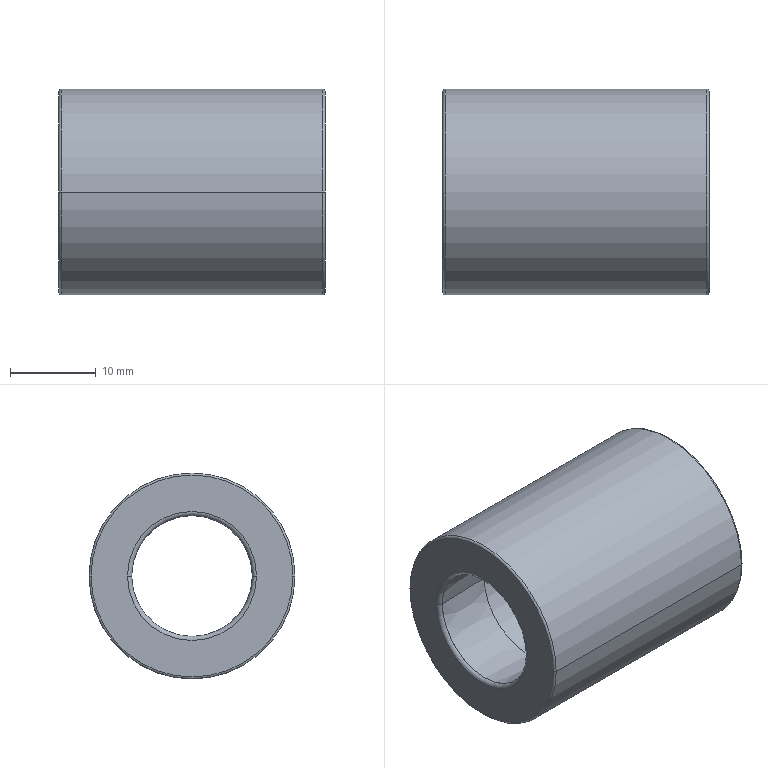Part | NX | 1 solid | 26 faces | box 31 x 24 x 24 mm | volume 8171 mm3 | torus 12 | cone 8 | cylinder 4 | plane 2 | commonest cylinder face diameters 16.674 x2 24 x2
STEP:
#1=CARTESIAN_POINT('',(-7.257,8.337,0.));
#2=VERTEX_POINT('',#1);
#3=CARTESIAN_POINT('',(-7.257,-8.337,0.));
#4=VERTEX_POINT('',#3);
#5=CARTESIAN_POINT('',(-7.257,0.,0.));
#6=DIRECTION('',(-1.,0.,0.));
#7=DIRECTION('',(0.,-1.,0.));
#8=AXIS2_PLACEMENT_3D('',#5,#6,#7);
#9=CIRCLE('',#8,8.337);
#10=EDGE_CURVE('',#2,#4,#9,.T.);
#11=ORIENTED_EDGE('',*,*,#10,.T.);
#12=CARTESIAN_POINT('',(7.257,-8.337,0.));
#13=VERTEX_POINT('',#12);
#14=CARTESIAN_POINT('',(0.,-8.337,0.));
#15=DIRECTION('',(1.,0.,0.));
#16=VECTOR('',#15,1000.);
#17=LINE('',#14,#16);
#18=EDGE_CURVE('',#4,#13,#17,.T.);
#19=ORIENTED_EDGE('',*,*,#18,.T.);
#20=CARTESIAN_POINT('',(7.257,8.337,0.));
#21=VERTEX_POINT('',#20);
#22=CARTESIAN_POINT('',(7.257,0.,0.));
#23=DIRECTION('',(1.,0.,0.));
#24=DIRECTION('',(0.,-1.,0.));
#25=AXIS2_PLACEMENT_3D('',#22,#23,#24);
#26=CIRCLE('',#25,8.337);
#27=EDGE_CURVE('',#13,#21,#26,.T.);
#28=ORIENTED_EDGE('',*,*,#27,.T.);
#29=CARTESIAN_POINT('',(0.,8.337,0.));
#30=DIRECTION('',(1.,0.,0.));
#31=VECTOR('',#30,1000.);
#32=LINE('',#29,#31);
#33=EDGE_CURVE('',#2,#21,#32,.T.);
#34=ORIENTED_EDGE('',*,*,#33,.F.);
#35=EDGE_LOOP('',(#11,#19,#28,#34));
#36=FACE_BOUND('',#35,.T.);
#37=CARTESIAN_POINT('',(0.,0.,0.));
#38=DIRECTION('',(1.,0.,0.));
#39=DIRECTION('',(0.,1.,0.));
#40=AXIS2_PLACEMENT_3D('',#37,#38,#39);
#41=CYLINDRICAL_SURFACE('',#40,8.337);
#42=ADVANCED_FACE('',(#36),#41,.F.);
#43=CARTESIAN_POINT('',(-15.02,7.033,0.));
#44=VERTEX_POINT('',#43);
#45=CARTESIAN_POINT('',(-15.02,-7.033,0.));
#46=VERTEX_POINT('',#45);
#47=CARTESIAN_POINT('',(-15.02,0.,0.));
#48=DIRECTION('',(-1.,0.,0.));
#49=DIRECTION('',(0.,0.,1.));
#50=AXIS2_PLACEMENT_3D('',#47,#48,#49);
#51=CIRCLE('',#50,7.033);
#52=EDGE_CURVE('',#44,#46,#51,.T.);
#53=ORIENTED_EDGE('',*,*,#52,.F.);
#54=CARTESIAN_POINT('',(-15.5,7.513,0.));
#55=VERTEX_POINT('',#54);
#56=CARTESIAN_POINT('',(-15.02,7.513,0.));
#57=DIRECTION('',(0.,0.,-1.));
#58=DIRECTION('',(-1.,0.,0.));
#59=AXIS2_PLACEMENT_3D('',#56,#57,#58);
#60=CIRCLE('',#59,0.48);
#61=EDGE_CURVE('',#55,#44,#60,.F.);
#62=ORIENTED_EDGE('',*,*,#61,.F.);
#63=CARTESIAN_POINT('',(-15.5,-7.513,0.));
#64=VERTEX_POINT('',#63);
#65=CARTESIAN_POINT('',(-15.5,0.,0.));
#66=DIRECTION('',(-1.,0.,0.));
#67=DIRECTION('',(0.,1.,0.));
#68=AXIS2_PLACEMENT_3D('',#65,#66,#67);
#69=CIRCLE('',#68,7.513);
#70=EDGE_CURVE('',#55,#64,#69,.T.);
#71=ORIENTED_EDGE('',*,*,#70,.T.);
#72=CARTESIAN_POINT('',(-15.02,-7.513,0.));
#73=DIRECTION('',(0.,0.,1.));
#74=DIRECTION('',(-1.,0.,0.));
#75=AXIS2_PLACEMENT_3D('',#72,#73,#74);
#76=CIRCLE('',#75,0.48);
#77=EDGE_CURVE('',#64,#46,#76,.F.);
#78=ORIENTED_EDGE('',*,*,#77,.T.);
#79=EDGE_LOOP('',(#53,#62,#71,#78));
#80=FACE_BOUND('',#79,.T.);
#81=CARTESIAN_POINT('',(-15.02,0.,0.));
#82=DIRECTION('',(-1.,0.,0.));
#83=DIRECTION('',(0.,1.,0.));
#84=AXIS2_PLACEMENT_3D('',#81,#82,#83);
#85=TOROIDAL_SURFACE('',#84,7.513,0.48);
#86=ADVANCED_FACE('',(#80),#85,.T.);
#87=CARTESIAN_POINT('',(15.02,-7.033,0.));
#88=VERTEX_POINT('',#87);
#89=CARTESIAN_POINT('',(15.02,7.033,0.));
#90=VERTEX_POINT('',#89);
#91=CARTESIAN_POINT('',(15.02,0.,0.));
#92=DIRECTION('',(-1.,0.,0.));
#93=DIRECTION('',(0.,0.,1.));
#94=AXIS2_PLACEMENT_3D('',#91,#92,#93);
#95=CIRCLE('',#94,7.033);
#96=EDGE_CURVE('',#88,#90,#95,.T.);
#97=ORIENTED_EDGE('',*,*,#96,.F.);
#98=CARTESIAN_POINT('',(15.005,-7.033,0.));
#99=VERTEX_POINT('',#98);
#100=CARTESIAN_POINT('',(15.02,-7.513,0.));
#101=DIRECTION('',(0.,0.,1.));
#102=DIRECTION('',(-1.,0.,0.));
#103=AXIS2_PLACEMENT_3D('',#100,#101,#102);
#104=CIRCLE('',#103,0.48);
#105=EDGE_CURVE('',#88,#99,#104,.T.);
#106=ORIENTED_EDGE('',*,*,#105,.T.);
#107=CARTESIAN_POINT('',(15.005,7.033,0.));
#108=VERTEX_POINT('',#107);
#109=CARTESIAN_POINT('',(15.005,0.,0.));
#110=DIRECTION('',(1.,0.,0.));
#111=DIRECTION('',(0.,-1.,0.));
#112=AXIS2_PLACEMENT_3D('',#109,#110,#111);
#113=CIRCLE('',#112,7.033);
#114=EDGE_CURVE('',#108,#99,#113,.T.);
#115=ORIENTED_EDGE('',*,*,#114,.F.);
#116=CARTESIAN_POINT('',(15.02,7.513,0.));
#117=DIRECTION('',(0.,0.,-1.));
#118=DIRECTION('',(-1.,0.,0.));
#119=AXIS2_PLACEMENT_3D('',#116,#117,#118);
#120=CIRCLE('',#119,0.48);
#121=EDGE_CURVE('',#90,#108,#120,.T.);
#122=ORIENTED_EDGE('',*,*,#121,.F.);
#123=EDGE_LOOP('',(#97,#106,#115,#122));
#124=FACE_BOUND('',#123,.T.);
#125=CARTESIAN_POINT('',(15.02,0.,0.));
#126=DIRECTION('',(-1.,0.,0.));
#127=DIRECTION('',(0.,1.,0.));
#128=AXIS2_PLACEMENT_3D('',#125,#126,#127);
#129=TOROIDAL_SURFACE('',#128,7.513,0.48);
#130=ADVANCED_FACE('',(#124),#129,.T.);
#131=ORIENTED_EDGE('',*,*,#27,.F.);
#132=CARTESIAN_POINT('',(7.881,-7.256,0.));
#133=VERTEX_POINT('',#132);
#134=CARTESIAN_POINT('',(7.569,-7.796,0.));
#135=DIRECTION('',(-0.5,-0.866,0.));
#136=VECTOR('',#135,1000.);
#137=LINE('',#134,#136);
#138=EDGE_CURVE('',#13,#133,#137,.F.);
#139=ORIENTED_EDGE('',*,*,#138,.T.);
#140=CARTESIAN_POINT('',(7.881,7.256,0.));
#141=VERTEX_POINT('',#140);
#142=CARTESIAN_POINT('',(7.881,0.,0.));
#143=DIRECTION('',(-1.,0.,0.));
#144=DIRECTION('',(0.,-1.,0.));
#145=AXIS2_PLACEMENT_3D('',#142,#143,#144);
#146=CIRCLE('',#145,7.256);
#147=EDGE_CURVE('',#141,#133,#146,.T.);
#148=ORIENTED_EDGE('',*,*,#147,.F.);
#149=CARTESIAN_POINT('',(7.569,7.796,0.));
#150=DIRECTION('',(-0.5,0.866,0.));
#151=VECTOR('',#150,1000.);
#152=LINE('',#149,#151);
#153=EDGE_CURVE('',#21,#141,#152,.F.);
#154=ORIENTED_EDGE('',*,*,#153,.F.);
#155=EDGE_LOOP('',(#131,#139,#148,#154));
#156=FACE_BOUND('',#155,.T.);
#157=CARTESIAN_POINT('',(7.569,0.,0.));
#158=DIRECTION('',(-1.,0.,0.));
#159=DIRECTION('',(0.,1.,0.));
#160=AXIS2_PLACEMENT_3D('',#157,#158,#159);
#161=CONICAL_SURFACE('',#160,7.796,1.047);
#162=ADVANCED_FACE('',(#156),#161,.F.);
#163=CARTESIAN_POINT('',(15.5,-11.76,0.));
#164=VERTEX_POINT('',#163);
#165=CARTESIAN_POINT('',(15.5,11.76,0.));
#166=VERTEX_POINT('',#165);
#167=CARTESIAN_POINT('',(15.5,0.,0.));
#168=DIRECTION('',(-1.,0.,0.));
#169=DIRECTION('',(0.,1.,0.));
#170=AXIS2_PLACEMENT_3D('',#167,#168,#169);
#171=CIRCLE('',#170,11.76);
#172=EDGE_CURVE('',#164,#166,#171,.T.);
#173=ORIENTED_EDGE('',*,*,#172,.F.);
#174=CARTESIAN_POINT('',(15.5,0.,0.));
#175=DIRECTION('',(-1.,0.,0.));
#176=DIRECTION('',(0.,1.,0.));
#177=AXIS2_PLACEMENT_3D('',#174,#175,#176);
#178=CIRCLE('',#177,11.76);
#179=EDGE_CURVE('',#166,#164,#178,.T.);
#180=ORIENTED_EDGE('',*,*,#179,.F.);
#181=EDGE_LOOP('',(#173,#180));
#182=FACE_BOUND('',#181,.T.);
#183=CARTESIAN_POINT('',(15.5,7.513,0.));
#184=VERTEX_POINT('',#183);
#185=CARTESIAN_POINT('',(15.5,-7.513,0.));
#186=VERTEX_POINT('',#185);
#187=CARTESIAN_POINT('',(15.5,0.,0.));
#188=DIRECTION('',(-1.,0.,0.));
#189=DIRECTION('',(0.,1.,0.));
#190=AXIS2_PLACEMENT_3D('',#187,#188,#189);
#191=CIRCLE('',#190,7.513);
#192=EDGE_CURVE('',#184,#186,#191,.T.);
#193=ORIENTED_EDGE('',*,*,#192,.T.);
#194=CARTESIAN_POINT('',(15.5,0.,0.));
#195=DIRECTION('',(-1.,0.,0.));
#196=DIRECTION('',(0.,1.,0.));
#197=AXIS2_PLACEMENT_3D('',#194,#195,#196);
#198=CIRCLE('',#197,7.513);
#199=EDGE_CURVE('',#186,#184,#198,.T.);
#200=ORIENTED_EDGE('',*,*,#199,.T.);
#201=EDGE_LOOP('',(#193,#200));
#202=FACE_BOUND('',#201,.T.);
#203=CARTESIAN_POINT('',(15.5,9.636,0.));
#204=DIRECTION('',(1.,0.,0.));
#205=DIRECTION('',(0.,1.,0.));
#206=AXIS2_PLACEMENT_3D('',#203,#204,#205);
#207=PLANE('',#206);
#208=ADVANCED_FACE('',(#182,#202),#207,.T.);
#209=ORIENTED_EDGE('',*,*,#172,.T.);
#210=CARTESIAN_POINT('',(15.26,12.,0.));
#211=VERTEX_POINT('',#210);
#212=CARTESIAN_POINT('',(15.26,11.76,0.));
#213=DIRECTION('',(0.,0.,-1.));
#214=DIRECTION('',(-1.,0.,0.));
#215=AXIS2_PLACEMENT_3D('',#212,#213,#214);
#216=CIRCLE('',#215,0.24);
#217=EDGE_CURVE('',#211,#166,#216,.T.);
#218=ORIENTED_EDGE('',*,*,#217,.F.);
#219=CARTESIAN_POINT('',(15.26,-12.,0.));
#220=VERTEX_POINT('',#219);
#221=CARTESIAN_POINT('',(15.26,0.,0.));
#222=DIRECTION('',(-1.,0.,0.));
#223=DIRECTION('',(0.,0.,-1.));
#224=AXIS2_PLACEMENT_3D('',#221,#222,#223);
#225=CIRCLE('',#224,12.);
#226=EDGE_CURVE('',#220,#211,#225,.T.);
#227=ORIENTED_EDGE('',*,*,#226,.F.);
#228=CARTESIAN_POINT('',(15.26,-11.76,0.));
#229=DIRECTION('',(0.,0.,1.));
#230=DIRECTION('',(-1.,0.,0.));
#231=AXIS2_PLACEMENT_3D('',#228,#229,#230);
#232=CIRCLE('',#231,0.24);
#233=EDGE_CURVE('',#220,#164,#232,.T.);
#234=ORIENTED_EDGE('',*,*,#233,.T.);
#235=EDGE_LOOP('',(#209,#218,#227,#234));
#236=FACE_BOUND('',#235,.T.);
#237=CARTESIAN_POINT('',(15.26,0.,0.));
#238=DIRECTION('',(-1.,0.,0.));
#239=DIRECTION('',(0.,1.,0.));
#240=AXIS2_PLACEMENT_3D('',#237,#238,#239);
#241=TOROIDAL_SURFACE('',#240,11.76,0.24);
#242=ADVANCED_FACE('',(#236),#241,.T.);
#243=CARTESIAN_POINT('',(7.881,0.,0.));
#244=DIRECTION('',(-1.,0.,0.));
#245=DIRECTION('',(0.,-1.,0.));
#246=AXIS2_PLACEMENT_3D('',#243,#244,#245);
#247=CIRCLE('',#246,7.256);
#248=EDGE_CURVE('',#133,#141,#247,.T.);
#249=ORIENTED_EDGE('',*,*,#248,.T.);
#250=CARTESIAN_POINT('',(11.443,7.144,0.));
#251=DIRECTION('',(-0.9995,0.03124,0.));
#252=VECTOR('',#251,1000.);
#253=LINE('',#250,#252);
#254=EDGE_CURVE('',#108,#141,#253,.T.);
#255=ORIENTED_EDGE('',*,*,#254,.F.);
#256=ORIENTED_EDGE('',*,*,#114,.T.);
#257=CARTESIAN_POINT('',(11.443,-7.144,0.));
#258=DIRECTION('',(-0.9995,-0.03124,0.));
#259=VECTOR('',#258,1000.);
#260=LINE('',#257,#259);
#261=EDGE_CURVE('',#99,#133,#260,.T.);
#262=ORIENTED_EDGE('',*,*,#261,.T.);
#263=EDGE_LOOP('',(#249,#255,#256,#262));
#264=FACE_BOUND('',#263,.T.);
#265=CARTESIAN_POINT('',(11.443,0.,0.));
#266=DIRECTION('',(-1.,0.,0.));
#267=DIRECTION('',(0.,1.,0.));
#268=AXIS2_PLACEMENT_3D('',#265,#266,#267);
#269=CONICAL_SURFACE('',#268,7.144,0.03124);
#270=ADVANCED_FACE('',(#264),#269,.F.);
#271=CARTESIAN_POINT('',(-15.26,12.,0.));
#272=VERTEX_POINT('',#271);
#273=CARTESIAN_POINT('',(-15.26,-12.,0.));
#274=VERTEX_POINT('',#273);
#275=CARTESIAN_POINT('',(-15.26,0.,0.));
#276=DIRECTION('',(1.,0.,0.));
#277=DIRECTION('',(0.,0.,-1.));
#278=AXIS2_PLACEMENT_3D('',#275,#276,#277);
#279=CIRCLE('',#278,12.);
#280=EDGE_CURVE('',#272,#274,#279,.T.);
#281=ORIENTED_EDGE('',*,*,#280,.T.);
#282=CARTESIAN_POINT('',(0.,-12.,0.));
#283=DIRECTION('',(1.,0.,0.));
#284=VECTOR('',#283,1000.);
#285=LINE('',#282,#284);
#286=EDGE_CURVE('',#220,#274,#285,.F.);
#287=ORIENTED_EDGE('',*,*,#286,.F.);
#288=ORIENTED_EDGE('',*,*,#226,.T.);
#289=CARTESIAN_POINT('',(0.,12.,0.));
#290=DIRECTION('',(1.,0.,0.));
#291=VECTOR('',#290,1000.);
#292=LINE('',#289,#291);
#293=EDGE_CURVE('',#211,#272,#292,.F.);
#294=ORIENTED_EDGE('',*,*,#293,.T.);
#295=EDGE_LOOP('',(#281,#287,#288,#294));
#296=FACE_BOUND('',#295,.T.);
#297=CARTESIAN_POINT('',(0.,0.,0.));
#298=DIRECTION('',(1.,0.,0.));
#299=DIRECTION('',(0.,1.,0.));
#300=AXIS2_PLACEMENT_3D('',#297,#298,#299);
#301=CYLINDRICAL_SURFACE('',#300,12.);
#302=ADVANCED_FACE('',(#296),#301,.T.);
#303=CARTESIAN_POINT('',(-7.881,-7.256,0.));
#304=VERTEX_POINT('',#303);
#305=CARTESIAN_POINT('',(-7.881,7.256,0.));
#306=VERTEX_POINT('',#305);
#307=CARTESIAN_POINT('',(-7.881,0.,0.));
#308=DIRECTION('',(-1.,0.,0.));
#309=DIRECTION('',(0.,1.,0.));
#310=AXIS2_PLACEMENT_3D('',#307,#308,#309);
#311=CIRCLE('',#310,7.256);
#312=EDGE_CURVE('',#304,#306,#311,.T.);
#313=ORIENTED_EDGE('',*,*,#312,.F.);
#314=CARTESIAN_POINT('',(-15.005,-7.033,0.));
#315=VERTEX_POINT('',#314);
#316=CARTESIAN_POINT('',(-11.443,-7.144,0.));
#317=DIRECTION('',(0.9995,-0.03124,0.));
#318=VECTOR('',#317,1000.);
#319=LINE('',#316,#318);
#320=EDGE_CURVE('',#304,#315,#319,.F.);
#321=ORIENTED_EDGE('',*,*,#320,.T.);
#322=CARTESIAN_POINT('',(-15.005,7.033,0.));
#323=VERTEX_POINT('',#322);
#324=CARTESIAN_POINT('',(-15.005,0.,0.));
#325=DIRECTION('',(-1.,0.,0.));
#326=DIRECTION('',(0.,0.,-1.));
#327=AXIS2_PLACEMENT_3D('',#324,#325,#326);
#328=CIRCLE('',#327,7.033);
#329=EDGE_CURVE('',#315,#323,#328,.T.);
#330=ORIENTED_EDGE('',*,*,#329,.T.);
#331=CARTESIAN_POINT('',(-11.443,7.144,0.));
#332=DIRECTION('',(0.9995,0.03124,0.));
#333=VECTOR('',#332,1000.);
#334=LINE('',#331,#333);
#335=EDGE_CURVE('',#306,#323,#334,.F.);
#336=ORIENTED_EDGE('',*,*,#335,.F.);
#337=EDGE_LOOP('',(#313,#321,#330,#336));
#338=FACE_BOUND('',#337,.T.);
#339=CARTESIAN_POINT('',(-11.443,0.,0.));
#340=DIRECTION('',(1.,0.,0.));
#341=DIRECTION('',(0.,-1.,0.));
#342=AXIS2_PLACEMENT_3D('',#339,#340,#341);
#343=CONICAL_SURFACE('',#342,7.144,0.03124);
#344=ADVANCED_FACE('',(#338),#343,.F.);
#345=CARTESIAN_POINT('',(-15.5,11.76,0.));
#346=VERTEX_POINT('',#345);
#347=CARTESIAN_POINT('',(-15.5,-11.76,0.));
#348=VERTEX_POINT('',#347);
#349=CARTESIAN_POINT('',(-15.5,0.,0.));
#350=DIRECTION('',(-1.,0.,0.));
#351=DIRECTION('',(0.,1.,0.));
#352=AXIS2_PLACEMENT_3D('',#349,#350,#351);
#353=CIRCLE('',#352,11.76);
#354=EDGE_CURVE('',#346,#348,#353,.T.);
#355=ORIENTED_EDGE('',*,*,#354,.F.);
#356=CARTESIAN_POINT('',(-15.26,11.76,0.));
#357=DIRECTION('',(0.,0.,-1.));
#358=DIRECTION('',(-1.,0.,0.));
#359=AXIS2_PLACEMENT_3D('',#356,#357,#358);
#360=CIRCLE('',#359,0.24);
#361=EDGE_CURVE('',#346,#272,#360,.T.);
#362=ORIENTED_EDGE('',*,*,#361,.T.);
#363=CARTESIAN_POINT('',(-15.26,0.,0.));
#364=DIRECTION('',(1.,0.,0.));
#365=DIRECTION('',(0.,0.,-1.));
#366=AXIS2_PLACEMENT_3D('',#363,#364,#365);
#367=CIRCLE('',#366,12.);
#368=EDGE_CURVE('',#274,#272,#367,.T.);
#369=ORIENTED_EDGE('',*,*,#368,.F.);
#370=CARTESIAN_POINT('',(-15.26,-11.76,0.));
#371=DIRECTION('',(0.,0.,1.));
#372=DIRECTION('',(-1.,0.,0.));
#373=AXIS2_PLACEMENT_3D('',#370,#371,#372);
#374=CIRCLE('',#373,0.24);
#375=EDGE_CURVE('',#348,#274,#374,.T.);
#376=ORIENTED_EDGE('',*,*,#375,.F.);
#377=EDGE_LOOP('',(#355,#362,#369,#376));
#378=FACE_BOUND('',#377,.T.);
#379=CARTESIAN_POINT('',(-15.26,0.,0.));
#380=DIRECTION('',(-1.,0.,0.));
#381=DIRECTION('',(0.,1.,0.));
#382=AXIS2_PLACEMENT_3D('',#379,#380,#381);
#383=TOROIDAL_SURFACE('',#382,11.76,0.24);
#384=ADVANCED_FACE('',(#378),#383,.T.);
#385=ORIENTED_EDGE('',*,*,#10,.F.);
#386=CARTESIAN_POINT('',(-7.569,7.796,0.));
#387=DIRECTION('',(0.5,0.866,0.));
#388=VECTOR('',#387,1000.);
#389=LINE('',#386,#388);
#390=EDGE_CURVE('',#306,#2,#389,.T.);
#391=ORIENTED_EDGE('',*,*,#390,.F.);
#392=CARTESIAN_POINT('',(-7.881,0.,0.));
#393=DIRECTION('',(-1.,0.,0.));
#394=DIRECTION('',(0.,1.,0.));
#395=AXIS2_PLACEMENT_3D('',#392,#393,#394);
#396=CIRCLE('',#395,7.256);
#397=EDGE_CURVE('',#306,#304,#396,.T.);
#398=ORIENTED_EDGE('',*,*,#397,.T.);
#399=CARTESIAN_POINT('',(-7.569,-7.796,0.));
#400=DIRECTION('',(0.5,-0.866,0.));
#401=VECTOR('',#400,1000.);
#402=LINE('',#399,#401);
#403=EDGE_CURVE('',#304,#4,#402,.T.);
#404=ORIENTED_EDGE('',*,*,#403,.T.);
#405=EDGE_LOOP('',(#385,#391,#398,#404));
#406=FACE_BOUND('',#405,.T.);
#407=CARTESIAN_POINT('',(-7.569,0.,0.));
#408=DIRECTION('',(1.,0.,0.));
#409=DIRECTION('',(0.,-1.,0.));
#410=AXIS2_PLACEMENT_3D('',#407,#408,#409);
#411=CONICAL_SURFACE('',#410,7.796,1.047);
#412=ADVANCED_FACE('',(#406),#411,.F.);
#413=ORIENTED_EDGE('',*,*,#354,.T.);
#414=CARTESIAN_POINT('',(-15.5,0.,0.));
#415=DIRECTION('',(-1.,0.,0.));
#416=DIRECTION('',(0.,1.,0.));
#417=AXIS2_PLACEMENT_3D('',#414,#415,#416);
#418=CIRCLE('',#417,11.76);
#419=EDGE_CURVE('',#348,#346,#418,.T.);
#420=ORIENTED_EDGE('',*,*,#419,.T.);
#421=EDGE_LOOP('',(#413,#420));
#422=FACE_BOUND('',#421,.T.);
#423=ORIENTED_EDGE('',*,*,#70,.F.);
#424=CARTESIAN_POINT('',(-15.5,0.,0.));
#425=DIRECTION('',(-1.,0.,0.));
#426=DIRECTION('',(0.,1.,0.));
#427=AXIS2_PLACEMENT_3D('',#424,#425,#426);
#428=CIRCLE('',#427,7.513);
#429=EDGE_CURVE('',#64,#55,#428,.T.);
#430=ORIENTED_EDGE('',*,*,#429,.F.);
#431=EDGE_LOOP('',(#423,#430));
#432=FACE_BOUND('',#431,.T.);
#433=CARTESIAN_POINT('',(-15.5,9.636,0.));
#434=DIRECTION('',(-1.,0.,0.));
#435=DIRECTION('',(0.,0.,1.));
#436=AXIS2_PLACEMENT_3D('',#433,#434,#435);
#437=PLANE('',#436);
#438=ADVANCED_FACE('',(#422,#432),#437,.T.);
#439=ORIENTED_EDGE('',*,*,#312,.T.);
#440=ORIENTED_EDGE('',*,*,#390,.T.);
#441=CARTESIAN_POINT('',(-7.257,0.,0.));
#442=DIRECTION('',(-1.,0.,0.));
#443=DIRECTION('',(0.,-1.,0.));
#444=AXIS2_PLACEMENT_3D('',#441,#442,#443);
#445=CIRCLE('',#444,8.337);
#446=EDGE_CURVE('',#4,#2,#445,.T.);
#447=ORIENTED_EDGE('',*,*,#446,.F.);
#448=ORIENTED_EDGE('',*,*,#403,.F.);
#449=EDGE_LOOP('',(#439,#440,#447,#448));
#450=FACE_BOUND('',#449,.T.);
#451=CARTESIAN_POINT('',(-7.569,0.,0.));
#452=DIRECTION('',(1.,0.,0.));
#453=DIRECTION('',(0.,-1.,0.));
#454=AXIS2_PLACEMENT_3D('',#451,#452,#453);
#455=CONICAL_SURFACE('',#454,7.796,1.047);
#456=ADVANCED_FACE('',(#450),#455,.F.);
#457=ORIENTED_EDGE('',*,*,#33,.T.);
#458=CARTESIAN_POINT('',(7.257,0.,0.));
#459=DIRECTION('',(1.,0.,0.));
#460=DIRECTION('',(0.,-1.,0.));
#461=AXIS2_PLACEMENT_3D('',#458,#459,#460);
#462=CIRCLE('',#461,8.337);
#463=EDGE_CURVE('',#21,#13,#462,.T.);
#464=ORIENTED_EDGE('',*,*,#463,.T.);
#465=ORIENTED_EDGE('',*,*,#18,.F.);
#466=ORIENTED_EDGE('',*,*,#446,.T.);
#467=EDGE_LOOP('',(#457,#464,#465,#466));
#468=FACE_BOUND('',#467,.T.);
#469=CARTESIAN_POINT('',(0.,0.,0.));
#470=DIRECTION('',(1.,0.,0.));
#471=DIRECTION('',(0.,1.,0.));
#472=AXIS2_PLACEMENT_3D('',#469,#470,#471);
#473=CYLINDRICAL_SURFACE('',#472,8.337);
#474=ADVANCED_FACE('',(#468),#473,.F.);
#475=CARTESIAN_POINT('',(15.26,0.,0.));
#476=DIRECTION('',(-1.,0.,0.));
#477=DIRECTION('',(0.,0.,-1.));
#478=AXIS2_PLACEMENT_3D('',#475,#476,#477);
#479=CIRCLE('',#478,12.);
#480=EDGE_CURVE('',#211,#220,#479,.T.);
#481=ORIENTED_EDGE('',*,*,#480,.T.);
#482=ORIENTED_EDGE('',*,*,#286,.T.);
#483=ORIENTED_EDGE('',*,*,#368,.T.);
#484=ORIENTED_EDGE('',*,*,#293,.F.);
#485=EDGE_LOOP('',(#481,#482,#483,#484));
#486=FACE_BOUND('',#485,.T.);
#487=CARTESIAN_POINT('',(0.,0.,0.));
#488=DIRECTION('',(1.,0.,0.));
#489=DIRECTION('',(0.,1.,0.));
#490=AXIS2_PLACEMENT_3D('',#487,#488,#489);
#491=CYLINDRICAL_SURFACE('',#490,12.);
#492=ADVANCED_FACE('',(#486),#491,.T.);
#493=ORIENTED_EDGE('',*,*,#248,.F.);
#494=ORIENTED_EDGE('',*,*,#138,.F.);
#495=ORIENTED_EDGE('',*,*,#463,.F.);
#496=ORIENTED_EDGE('',*,*,#153,.T.);
#497=EDGE_LOOP('',(#493,#494,#495,#496));
#498=FACE_BOUND('',#497,.T.);
#499=CARTESIAN_POINT('',(7.569,0.,0.));
#500=DIRECTION('',(-1.,0.,0.));
#501=DIRECTION('',(0.,1.,0.));
#502=AXIS2_PLACEMENT_3D('',#499,#500,#501);
#503=CONICAL_SURFACE('',#502,7.796,1.047);
#504=ADVANCED_FACE('',(#498),#503,.F.);
#505=ORIENTED_EDGE('',*,*,#254,.T.);
#506=ORIENTED_EDGE('',*,*,#147,.T.);
#507=ORIENTED_EDGE('',*,*,#261,.F.);
#508=CARTESIAN_POINT('',(15.005,0.,0.));
#509=DIRECTION('',(1.,0.,0.));
#510=DIRECTION('',(0.,-1.,0.));
#511=AXIS2_PLACEMENT_3D('',#508,#509,#510);
#512=CIRCLE('',#511,7.033);
#513=EDGE_CURVE('',#99,#108,#512,.T.);
#514=ORIENTED_EDGE('',*,*,#513,.T.);
#515=EDGE_LOOP('',(#505,#506,#507,#514));
#516=FACE_BOUND('',#515,.T.);
#517=CARTESIAN_POINT('',(11.443,0.,0.));
#518=DIRECTION('',(-1.,0.,0.));
#519=DIRECTION('',(0.,1.,0.));
#520=AXIS2_PLACEMENT_3D('',#517,#518,#519);
#521=CONICAL_SURFACE('',#520,7.144,0.03124);
#522=ADVANCED_FACE('',(#516),#521,.F.);
#523=CARTESIAN_POINT('',(-15.005,0.,0.));
#524=DIRECTION('',(-1.,0.,0.));
#525=DIRECTION('',(0.,0.,-1.));
#526=AXIS2_PLACEMENT_3D('',#523,#524,#525);
#527=CIRCLE('',#526,7.033);
#528=EDGE_CURVE('',#323,#315,#527,.T.);
#529=ORIENTED_EDGE('',*,*,#528,.T.);
#530=ORIENTED_EDGE('',*,*,#320,.F.);
#531=ORIENTED_EDGE('',*,*,#397,.F.);
#532=ORIENTED_EDGE('',*,*,#335,.T.);
#533=EDGE_LOOP('',(#529,#530,#531,#532));
#534=FACE_BOUND('',#533,.T.);
#535=CARTESIAN_POINT('',(-11.443,0.,0.));
#536=DIRECTION('',(1.,0.,0.));
#537=DIRECTION('',(0.,-1.,0.));
#538=AXIS2_PLACEMENT_3D('',#535,#536,#537);
#539=CONICAL_SURFACE('',#538,7.144,0.03124);
#540=ADVANCED_FACE('',(#534),#539,.F.);
#541=ORIENTED_EDGE('',*,*,#480,.F.);
#542=ORIENTED_EDGE('',*,*,#217,.T.);
#543=ORIENTED_EDGE('',*,*,#179,.T.);
#544=ORIENTED_EDGE('',*,*,#233,.F.);
#545=EDGE_LOOP('',(#541,#542,#543,#544));
#546=FACE_BOUND('',#545,.T.);
#547=CARTESIAN_POINT('',(15.26,0.,0.));
#548=DIRECTION('',(-1.,0.,0.));
#549=DIRECTION('',(0.,1.,0.));
#550=AXIS2_PLACEMENT_3D('',#547,#548,#549);
#551=TOROIDAL_SURFACE('',#550,11.76,0.24);
#552=ADVANCED_FACE('',(#546),#551,.T.);
#553=ORIENTED_EDGE('',*,*,#280,.F.);
#554=ORIENTED_EDGE('',*,*,#361,.F.);
#555=ORIENTED_EDGE('',*,*,#419,.F.);
#556=ORIENTED_EDGE('',*,*,#375,.T.);
#557=EDGE_LOOP('',(#553,#554,#555,#556));
#558=FACE_BOUND('',#557,.T.);
#559=CARTESIAN_POINT('',(-15.26,0.,0.));
#560=DIRECTION('',(-1.,0.,0.));
#561=DIRECTION('',(0.,1.,0.));
#562=AXIS2_PLACEMENT_3D('',#559,#560,#561);
#563=TOROIDAL_SURFACE('',#562,11.76,0.24);
#564=ADVANCED_FACE('',(#558),#563,.T.);
#565=CARTESIAN_POINT('',(-15.02,0.,0.));
#566=DIRECTION('',(-1.,0.,0.));
#567=DIRECTION('',(0.,0.,1.));
#568=AXIS2_PLACEMENT_3D('',#565,#566,#567);
#569=CIRCLE('',#568,7.033);
#570=EDGE_CURVE('',#46,#44,#569,.T.);
#571=ORIENTED_EDGE('',*,*,#570,.F.);
#572=ORIENTED_EDGE('',*,*,#77,.F.);
#573=ORIENTED_EDGE('',*,*,#429,.T.);
#574=ORIENTED_EDGE('',*,*,#61,.T.);
#575=EDGE_LOOP('',(#571,#572,#573,#574));
#576=FACE_BOUND('',#575,.T.);
#577=CARTESIAN_POINT('',(-15.02,0.,0.));
#578=DIRECTION('',(-1.,0.,0.));
#579=DIRECTION('',(0.,1.,0.));
#580=AXIS2_PLACEMENT_3D('',#577,#578,#579);
#581=TOROIDAL_SURFACE('',#580,7.513,0.48);
#582=ADVANCED_FACE('',(#576),#581,.T.);
#583=CARTESIAN_POINT('',(15.02,0.,0.));
#584=DIRECTION('',(-1.,0.,0.));
#585=DIRECTION('',(0.,0.,1.));
#586=AXIS2_PLACEMENT_3D('',#583,#584,#585);
#587=CIRCLE('',#586,7.033);
#588=EDGE_CURVE('',#90,#88,#587,.T.);
#589=ORIENTED_EDGE('',*,*,#588,.F.);
#590=ORIENTED_EDGE('',*,*,#121,.T.);
#591=ORIENTED_EDGE('',*,*,#513,.F.);
#592=ORIENTED_EDGE('',*,*,#105,.F.);
#593=EDGE_LOOP('',(#589,#590,#591,#592));
#594=FACE_BOUND('',#593,.T.);
#595=CARTESIAN_POINT('',(15.02,0.,0.));
#596=DIRECTION('',(-1.,0.,0.));
#597=DIRECTION('',(0.,1.,0.));
#598=AXIS2_PLACEMENT_3D('',#595,#596,#597);
#599=TOROIDAL_SURFACE('',#598,7.513,0.48);
#600=ADVANCED_FACE('',(#594),#599,.T.);
#601=CARTESIAN_POINT('',(15.02,7.513,0.));
#602=DIRECTION('',(0.,0.,-1.));
#603=DIRECTION('',(-1.,0.,0.));
#604=AXIS2_PLACEMENT_3D('',#601,#602,#603);
#605=CIRCLE('',#604,0.48);
#606=EDGE_CURVE('',#90,#184,#605,.F.);
#607=ORIENTED_EDGE('',*,*,#606,.F.);
#608=ORIENTED_EDGE('',*,*,#588,.T.);
#609=CARTESIAN_POINT('',(15.02,-7.513,0.));
#610=DIRECTION('',(0.,0.,1.));
#611=DIRECTION('',(-1.,0.,0.));
#612=AXIS2_PLACEMENT_3D('',#609,#610,#611);
#613=CIRCLE('',#612,0.48);
#614=EDGE_CURVE('',#88,#186,#613,.F.);
#615=ORIENTED_EDGE('',*,*,#614,.T.);
#616=ORIENTED_EDGE('',*,*,#192,.F.);
#617=EDGE_LOOP('',(#607,#608,#615,#616));
#618=FACE_BOUND('',#617,.T.);
#619=CARTESIAN_POINT('',(15.02,0.,0.));
#620=DIRECTION('',(-1.,0.,0.));
#621=DIRECTION('',(0.,1.,0.));
#622=AXIS2_PLACEMENT_3D('',#619,#620,#621);
#623=TOROIDAL_SURFACE('',#622,7.513,0.48);
#624=ADVANCED_FACE('',(#618),#623,.T.);
#625=CARTESIAN_POINT('',(-15.02,-7.513,0.));
#626=DIRECTION('',(0.,0.,1.));
#627=DIRECTION('',(-1.,0.,0.));
#628=AXIS2_PLACEMENT_3D('',#625,#626,#627);
#629=CIRCLE('',#628,0.48);
#630=EDGE_CURVE('',#315,#46,#629,.T.);
#631=ORIENTED_EDGE('',*,*,#630,.T.);
#632=ORIENTED_EDGE('',*,*,#570,.T.);
#633=CARTESIAN_POINT('',(-15.02,7.513,0.));
#634=DIRECTION('',(0.,0.,-1.));
#635=DIRECTION('',(-1.,0.,0.));
#636=AXIS2_PLACEMENT_3D('',#633,#634,#635);
#637=CIRCLE('',#636,0.48);
#638=EDGE_CURVE('',#323,#44,#637,.T.);
#639=ORIENTED_EDGE('',*,*,#638,.F.);
#640=ORIENTED_EDGE('',*,*,#329,.F.);
#641=EDGE_LOOP('',(#631,#632,#639,#640));
#642=FACE_BOUND('',#641,.T.);
#643=CARTESIAN_POINT('',(-15.02,0.,0.));
#644=DIRECTION('',(-1.,0.,0.));
#645=DIRECTION('',(0.,1.,0.));
#646=AXIS2_PLACEMENT_3D('',#643,#644,#645);
#647=TOROIDAL_SURFACE('',#646,7.513,0.48);
#648=ADVANCED_FACE('',(#642),#647,.T.);
#649=ORIENTED_EDGE('',*,*,#614,.F.);
#650=ORIENTED_EDGE('',*,*,#96,.T.);
#651=ORIENTED_EDGE('',*,*,#606,.T.);
#652=ORIENTED_EDGE('',*,*,#199,.F.);
#653=EDGE_LOOP('',(#649,#650,#651,#652));
#654=FACE_BOUND('',#653,.T.);
#655=CARTESIAN_POINT('',(15.02,0.,0.));
#656=DIRECTION('',(-1.,0.,0.));
#657=DIRECTION('',(0.,1.,0.));
#658=AXIS2_PLACEMENT_3D('',#655,#656,#657);
#659=TOROIDAL_SURFACE('',#658,7.513,0.48);
#660=ADVANCED_FACE('',(#654),#659,.T.);
#661=ORIENTED_EDGE('',*,*,#638,.T.);
#662=ORIENTED_EDGE('',*,*,#52,.T.);
#663=ORIENTED_EDGE('',*,*,#630,.F.);
#664=ORIENTED_EDGE('',*,*,#528,.F.);
#665=EDGE_LOOP('',(#661,#662,#663,#664));
#666=FACE_BOUND('',#665,.T.);
#667=CARTESIAN_POINT('',(-15.02,0.,0.));
#668=DIRECTION('',(-1.,0.,0.));
#669=DIRECTION('',(0.,1.,0.));
#670=AXIS2_PLACEMENT_3D('',#667,#668,#669);
#671=TOROIDAL_SURFACE('',#670,7.513,0.48);
#672=ADVANCED_FACE('',(#666),#671,.T.);
#673=CLOSED_SHELL('',(#42,#86,#130,#162,#208,#242,#270,#302,#344,#384,#412,#438,#456,#474,#492,#504,#522,#540,#552,#564,#582,#600,#624,#648,#660,#672));
#674=MANIFOLD_SOLID_BREP('',#673);
#675=(LENGTH_UNIT()NAMED_UNIT(*)SI_UNIT(.MILLI.,.METRE.));
#676=UNCERTAINTY_MEASURE_WITH_UNIT(LENGTH_MEASURE(0.00001),#675,'','');
#677=(NAMED_UNIT(*)PLANE_ANGLE_UNIT()SI_UNIT($,.RADIAN.));
#678=(NAMED_UNIT(*)SI_UNIT($,.STERADIAN.)SOLID_ANGLE_UNIT());
#679=(GEOMETRIC_REPRESENTATION_CONTEXT(3)GLOBAL_UNCERTAINTY_ASSIGNED_CONTEXT((#676))GLOBAL_UNIT_ASSIGNED_CONTEXT((#675,#677,#678))REPRESENTATION_CONTEXT('',''));
#680=ADVANCED_BREP_SHAPE_REPRESENTATION('',(#674),#679);